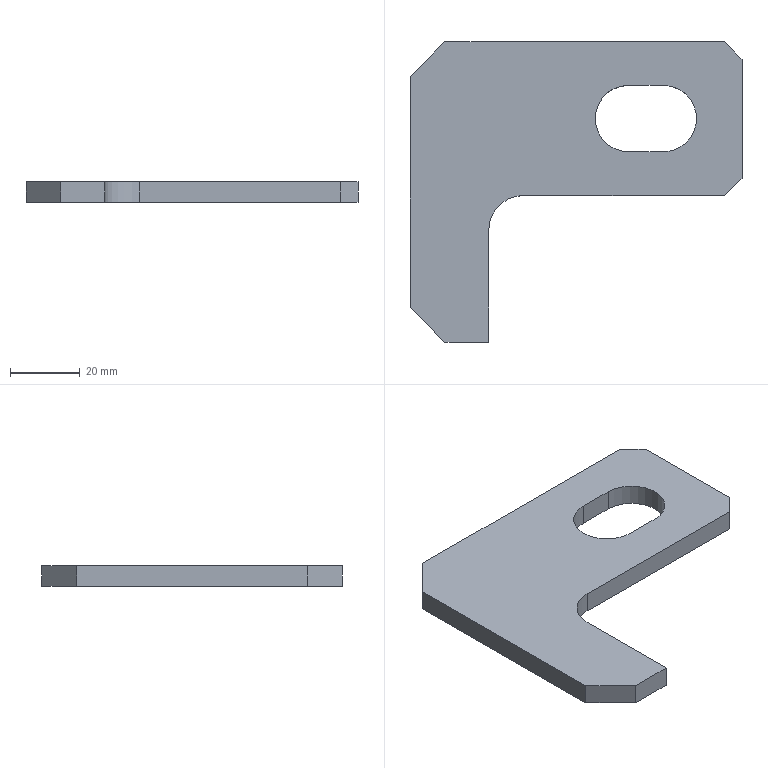Part | STEP file | 筋Plate-100×50-5 | 1 solid | 18 faces | box 95 x 86 x 6 mm | volume 27288 mm3 | plane 14 | cylinder 4 | commonest cylinder face diameters 19 x3 20 x1
STEP:
#1=CARTESIAN_POINT('',(0.,0.,0.));
#2=DIRECTION('',(0.,0.,1.));
#3=DIRECTION('',(1.,0.,0.));
#4=AXIS2_PLACEMENT_3D('',#1,#2,#3);
#5=CARTESIAN_POINT('',(15.,30.5,3.));
#6=VERTEX_POINT('',#5);
#7=CARTESIAN_POINT('',(15.,30.5,-3.));
#8=VERTEX_POINT('',#7);
#9=CARTESIAN_POINT('',(15.,30.5,-3.));
#10=DIRECTION('',(0.,0.,-1.));
#11=VECTOR('',#10,1.);
#12=LINE('',#9,#11);
#13=CARTESIAN_POINT('',(15.,21.,-3.));
#14=DIRECTION('',(0.,0.,-1.));
#15=DIRECTION('',(-1.,0.,0.));
#16=AXIS2_PLACEMENT_3D('',#13,#14,#15);
#17=CYLINDRICAL_SURFACE('',#16,9.5);
#18=CARTESIAN_POINT('',(1.571,0.));
#19=DIRECTION('',(0.,1.));
#20=VECTOR('',#19,1.);
#21=LINE('',#18,#20);
#22=(GEOMETRIC_REPRESENTATION_CONTEXT(2)PARAMETRIC_REPRESENTATION_CONTEXT()REPRESENTATION_CONTEXT('',''));
#23=DEFINITIONAL_REPRESENTATION('',(#21),#22);
#24=PCURVE('',#17,#23);
#25=CARTESIAN_POINT('',(15.,30.5,-3.));
#26=DIRECTION('',(0.,1.,0.));
#27=DIRECTION('',(-1.,0.,0.));
#28=AXIS2_PLACEMENT_3D('',#25,#26,#27);
#29=PLANE('',#28);
#30=CARTESIAN_POINT('',(0.,0.));
#31=DIRECTION('',(0.,-1.));
#32=VECTOR('',#31,1.);
#33=LINE('',#30,#32);
#34=(GEOMETRIC_REPRESENTATION_CONTEXT(2)PARAMETRIC_REPRESENTATION_CONTEXT()REPRESENTATION_CONTEXT('',''));
#35=DEFINITIONAL_REPRESENTATION('',(#33),#34);
#36=PCURVE('',#29,#35);
#37=SURFACE_CURVE('',#12,(#24,#36),.PCURVE_S1.);
#38=EDGE_CURVE('',#6,#8,#37,.T.);
#39=ORIENTED_EDGE('',*,*,#38,.T.);
#40=CARTESIAN_POINT('',(5.5,21.,-3.));
#41=VERTEX_POINT('',#40);
#42=CARTESIAN_POINT('',(15.,21.,-3.));
#43=DIRECTION('',(0.,0.,-1.));
#44=DIRECTION('',(-1.,0.,0.));
#45=AXIS2_PLACEMENT_3D('',#42,#43,#44);
#46=CIRCLE('',#45,9.5);
#47=CARTESIAN_POINT('',(0.,0.));
#48=DIRECTION('',(1.,0.));
#49=VECTOR('',#48,1.);
#50=LINE('',#47,#49);
#51=(GEOMETRIC_REPRESENTATION_CONTEXT(2)PARAMETRIC_REPRESENTATION_CONTEXT()REPRESENTATION_CONTEXT('',''));
#52=DEFINITIONAL_REPRESENTATION('',(#50),#51);
#53=PCURVE('',#17,#52);
#54=CARTESIAN_POINT('',(0.,0.,-3.));
#55=DIRECTION('',(0.,0.,1.));
#56=DIRECTION('',(1.,0.,0.));
#57=AXIS2_PLACEMENT_3D('',#54,#55,#56);
#58=PLANE('',#57);
#59=CARTESIAN_POINT('',(5.5,21.));
#60=CARTESIAN_POINT('',(5.5,37.454));
#61=CARTESIAN_POINT('',(19.75,29.227));
#62=CARTESIAN_POINT('',(34.,21.));
#63=CARTESIAN_POINT('',(19.75,12.773));
#64=CARTESIAN_POINT('',(5.5,4.546));
#65=CARTESIAN_POINT('',(5.5,21.));
#66=(BOUNDED_CURVE()B_SPLINE_CURVE(2,(#59,#60,#61,#62,#63,#64,#65),.UNSPECIFIED.,.T.,.F.)B_SPLINE_CURVE_WITH_KNOTS((1,2,2,2,2,1),(-2.094,0.,2.094,4.189,6.283,8.378),.UNSPECIFIED.)CURVE()GEOMETRIC_REPRESENTATION_ITEM()RATIONAL_B_SPLINE_CURVE((1.,0.5,1.,0.5,1.,0.5,1.))REPRESENTATION_ITEM(''));
#67=(GEOMETRIC_REPRESENTATION_CONTEXT(2)PARAMETRIC_REPRESENTATION_CONTEXT()REPRESENTATION_CONTEXT('',''));
#68=DEFINITIONAL_REPRESENTATION('',(#66),#67);
#69=PCURVE('',#58,#68);
#70=SURFACE_CURVE('',#46,(#53,#69),.PCURVE_S1.);
#71=EDGE_CURVE('',#41,#8,#70,.T.);
#72=ORIENTED_EDGE('',*,*,#71,.F.);
#73=CARTESIAN_POINT('',(5.5,21.,3.));
#74=VERTEX_POINT('',#73);
#75=CARTESIAN_POINT('',(5.5,21.,-3.));
#76=DIRECTION('',(0.,0.,-1.));
#77=VECTOR('',#76,1.);
#78=LINE('',#75,#77);
#79=CARTESIAN_POINT('',(0.,0.));
#80=DIRECTION('',(0.,1.));
#81=VECTOR('',#80,1.);
#82=LINE('',#79,#81);
#83=(GEOMETRIC_REPRESENTATION_CONTEXT(2)PARAMETRIC_REPRESENTATION_CONTEXT()REPRESENTATION_CONTEXT('',''));
#84=DEFINITIONAL_REPRESENTATION('',(#82),#83);
#85=PCURVE('',#17,#84);
#86=CARTESIAN_POINT('',(15.,21.,-3.));
#87=DIRECTION('',(0.,0.,-1.));
#88=DIRECTION('',(-1.,0.,0.));
#89=AXIS2_PLACEMENT_3D('',#86,#87,#88);
#90=CYLINDRICAL_SURFACE('',#89,9.5);
#91=CARTESIAN_POINT('',(6.283,0.));
#92=DIRECTION('',(0.,1.));
#93=VECTOR('',#92,1.);
#94=LINE('',#91,#93);
#95=(GEOMETRIC_REPRESENTATION_CONTEXT(2)PARAMETRIC_REPRESENTATION_CONTEXT()REPRESENTATION_CONTEXT('',''));
#96=DEFINITIONAL_REPRESENTATION('',(#94),#95);
#97=PCURVE('',#90,#96);
#98=SURFACE_CURVE('',#78,(#85,#97),.PCURVE_S1.);
#99=EDGE_CURVE('',#74,#41,#98,.T.);
#100=ORIENTED_EDGE('',*,*,#99,.F.);
#101=CARTESIAN_POINT('',(15.,21.,3.));
#102=DIRECTION('',(0.,0.,1.));
#103=DIRECTION('',(1.,0.,0.));
#104=AXIS2_PLACEMENT_3D('',#101,#102,#103);
#105=CIRCLE('',#104,9.5);
#106=CARTESIAN_POINT('',(3.142,-6.));
#107=DIRECTION('',(-1.,0.));
#108=VECTOR('',#107,1.);
#109=LINE('',#106,#108);
#110=(GEOMETRIC_REPRESENTATION_CONTEXT(2)PARAMETRIC_REPRESENTATION_CONTEXT()REPRESENTATION_CONTEXT('',''));
#111=DEFINITIONAL_REPRESENTATION('',(#109),#110);
#112=PCURVE('',#17,#111);
#113=CARTESIAN_POINT('',(0.,0.,3.));
#114=DIRECTION('',(0.,0.,1.));
#115=DIRECTION('',(1.,0.,0.));
#116=AXIS2_PLACEMENT_3D('',#113,#114,#115);
#117=PLANE('',#116);
#118=CARTESIAN_POINT('',(15.,21.));
#119=DIRECTION('',(1.,0.));
#120=AXIS2_PLACEMENT_2D('',#118,#119);
#121=CIRCLE('',#120,9.5);
#122=(GEOMETRIC_REPRESENTATION_CONTEXT(2)PARAMETRIC_REPRESENTATION_CONTEXT()REPRESENTATION_CONTEXT('',''));
#123=DEFINITIONAL_REPRESENTATION('',(#121),#122);
#124=PCURVE('',#117,#123);
#125=SURFACE_CURVE('',#105,(#112,#124),.PCURVE_S1.);
#126=EDGE_CURVE('',#6,#74,#125,.T.);
#127=ORIENTED_EDGE('',*,*,#126,.F.);
#128=EDGE_LOOP('',(#39,#72,#100,#127));
#129=FACE_BOUND('',#128,.F.);
#130=ADVANCED_FACE('',(#129),#17,.F.);
#131=CARTESIAN_POINT('',(47.5,38.,3.));
#132=VERTEX_POINT('',#131);
#133=CARTESIAN_POINT('',(47.5,4.,3.));
#134=VERTEX_POINT('',#133);
#135=CARTESIAN_POINT('',(47.5,0.,3.));
#136=DIRECTION('',(0.,-1.,0.));
#137=VECTOR('',#136,1.);
#138=LINE('',#135,#137);
#139=CARTESIAN_POINT('',(47.5,0.,3.));
#140=DIRECTION('',(1.,0.,0.));
#141=DIRECTION('',(0.,1.,0.));
#142=AXIS2_PLACEMENT_3D('',#139,#140,#141);
#143=PLANE('',#142);
#144=CARTESIAN_POINT('',(0.,0.));
#145=DIRECTION('',(-1.,0.));
#146=VECTOR('',#145,1.);
#147=LINE('',#144,#146);
#148=(GEOMETRIC_REPRESENTATION_CONTEXT(2)PARAMETRIC_REPRESENTATION_CONTEXT()REPRESENTATION_CONTEXT('',''));
#149=DEFINITIONAL_REPRESENTATION('',(#147),#148);
#150=PCURVE('',#143,#149);
#151=CARTESIAN_POINT('',(47.5,0.));
#152=DIRECTION('',(0.,-1.));
#153=VECTOR('',#152,1.);
#154=LINE('',#151,#153);
#155=(GEOMETRIC_REPRESENTATION_CONTEXT(2)PARAMETRIC_REPRESENTATION_CONTEXT()REPRESENTATION_CONTEXT('',''));
#156=DEFINITIONAL_REPRESENTATION('',(#154),#155);
#157=PCURVE('',#117,#156);
#158=SURFACE_CURVE('',#138,(#150,#157),.PCURVE_S1.);
#159=EDGE_CURVE('',#132,#134,#158,.T.);
#160=ORIENTED_EDGE('',*,*,#159,.T.);
#161=CARTESIAN_POINT('',(47.5,4.,-3.));
#162=VERTEX_POINT('',#161);
#163=CARTESIAN_POINT('',(47.5,4.,-3.));
#164=DIRECTION('',(0.,0.,-1.));
#165=VECTOR('',#164,1.);
#166=LINE('',#163,#165);
#167=CARTESIAN_POINT('',(4.,-6.));
#168=DIRECTION('',(0.,-1.));
#169=VECTOR('',#168,1.);
#170=LINE('',#167,#169);
#171=(GEOMETRIC_REPRESENTATION_CONTEXT(2)PARAMETRIC_REPRESENTATION_CONTEXT()REPRESENTATION_CONTEXT('',''));
#172=DEFINITIONAL_REPRESENTATION('',(#170),#171);
#173=PCURVE('',#143,#172);
#174=CARTESIAN_POINT('',(42.5,-1.,-3.));
#175=DIRECTION('',(0.7071,-0.7071,0.));
#176=DIRECTION('',(0.,0.,-1.));
#177=AXIS2_PLACEMENT_3D('',#174,#175,#176);
#178=PLANE('',#177);
#179=CARTESIAN_POINT('',(0.,7.071));
#180=DIRECTION('',(1.,0.));
#181=VECTOR('',#180,1.);
#182=LINE('',#179,#181);
#183=(GEOMETRIC_REPRESENTATION_CONTEXT(2)PARAMETRIC_REPRESENTATION_CONTEXT()REPRESENTATION_CONTEXT('',''));
#184=DEFINITIONAL_REPRESENTATION('',(#182),#183);
#185=PCURVE('',#178,#184);
#186=SURFACE_CURVE('',#166,(#173,#185),.PCURVE_S1.);
#187=EDGE_CURVE('',#134,#162,#186,.T.);
#188=ORIENTED_EDGE('',*,*,#187,.T.);
#189=CARTESIAN_POINT('',(47.5,38.,-3.));
#190=VERTEX_POINT('',#189);
#191=CARTESIAN_POINT('',(47.5,0.,-3.));
#192=DIRECTION('',(0.,-1.,0.));
#193=VECTOR('',#192,1.);
#194=LINE('',#191,#193);
#195=CARTESIAN_POINT('',(0.,-6.));
#196=DIRECTION('',(-1.,0.));
#197=VECTOR('',#196,1.);
#198=LINE('',#195,#197);
#199=(GEOMETRIC_REPRESENTATION_CONTEXT(2)PARAMETRIC_REPRESENTATION_CONTEXT()REPRESENTATION_CONTEXT('',''));
#200=DEFINITIONAL_REPRESENTATION('',(#198),#199);
#201=PCURVE('',#143,#200);
#202=CARTESIAN_POINT('',(47.5,0.));
#203=DIRECTION('',(0.,-1.));
#204=VECTOR('',#203,1.);
#205=LINE('',#202,#204);
#206=(GEOMETRIC_REPRESENTATION_CONTEXT(2)PARAMETRIC_REPRESENTATION_CONTEXT()REPRESENTATION_CONTEXT('',''));
#207=DEFINITIONAL_REPRESENTATION('',(#205),#206);
#208=PCURVE('',#58,#207);
#209=SURFACE_CURVE('',#194,(#201,#208),.PCURVE_S1.);
#210=EDGE_CURVE('',#190,#162,#209,.T.);
#211=ORIENTED_EDGE('',*,*,#210,.F.);
#212=CARTESIAN_POINT('',(47.5,38.,3.));
#213=DIRECTION('',(0.,0.,1.));
#214=VECTOR('',#213,1.);
#215=LINE('',#212,#214);
#216=CARTESIAN_POINT('',(38.,0.));
#217=DIRECTION('',(0.,1.));
#218=VECTOR('',#217,1.);
#219=LINE('',#216,#218);
#220=(GEOMETRIC_REPRESENTATION_CONTEXT(2)PARAMETRIC_REPRESENTATION_CONTEXT()REPRESENTATION_CONTEXT('',''));
#221=DEFINITIONAL_REPRESENTATION('',(#219),#220);
#222=PCURVE('',#143,#221);
#223=CARTESIAN_POINT('',(42.5,43.,3.));
#224=DIRECTION('',(-0.7071,-0.7071,0.));
#225=DIRECTION('',(0.,0.,-1.));
#226=AXIS2_PLACEMENT_3D('',#223,#224,#225);
#227=PLANE('',#226);
#228=CARTESIAN_POINT('',(0.,7.071));
#229=DIRECTION('',(-1.,0.));
#230=VECTOR('',#229,1.);
#231=LINE('',#228,#230);
#232=(GEOMETRIC_REPRESENTATION_CONTEXT(2)PARAMETRIC_REPRESENTATION_CONTEXT()REPRESENTATION_CONTEXT('',''));
#233=DEFINITIONAL_REPRESENTATION('',(#231),#232);
#234=PCURVE('',#227,#233);
#235=SURFACE_CURVE('',#215,(#222,#234),.PCURVE_S1.);
#236=EDGE_CURVE('',#190,#132,#235,.T.);
#237=ORIENTED_EDGE('',*,*,#236,.T.);
#238=EDGE_LOOP('',(#160,#188,#211,#237));
#239=FACE_BOUND('',#238,.T.);
#240=ADVANCED_FACE('',(#239),#143,.T.);
#241=CARTESIAN_POINT('',(-37.5,43.,3.));
#242=VERTEX_POINT('',#241);
#243=CARTESIAN_POINT('',(42.5,43.,3.));
#244=VERTEX_POINT('',#243);
#245=CARTESIAN_POINT('',(0.,43.,3.));
#246=DIRECTION('',(1.,0.,0.));
#247=VECTOR('',#246,1.);
#248=LINE('',#245,#247);
#249=CARTESIAN_POINT('',(0.,43.,3.));
#250=DIRECTION('',(0.,1.,0.));
#251=DIRECTION('',(0.,0.,1.));
#252=AXIS2_PLACEMENT_3D('',#249,#250,#251);
#253=PLANE('',#252);
#254=CARTESIAN_POINT('',(0.,0.));
#255=DIRECTION('',(0.,1.));
#256=VECTOR('',#255,1.);
#257=LINE('',#254,#256);
#258=(GEOMETRIC_REPRESENTATION_CONTEXT(2)PARAMETRIC_REPRESENTATION_CONTEXT()REPRESENTATION_CONTEXT('',''));
#259=DEFINITIONAL_REPRESENTATION('',(#257),#258);
#260=PCURVE('',#253,#259);
#261=CARTESIAN_POINT('',(0.,43.));
#262=DIRECTION('',(1.,0.));
#263=VECTOR('',#262,1.);
#264=LINE('',#261,#263);
#265=(GEOMETRIC_REPRESENTATION_CONTEXT(2)PARAMETRIC_REPRESENTATION_CONTEXT()REPRESENTATION_CONTEXT('',''));
#266=DEFINITIONAL_REPRESENTATION('',(#264),#265);
#267=PCURVE('',#117,#266);
#268=SURFACE_CURVE('',#248,(#260,#267),.PCURVE_S1.);
#269=EDGE_CURVE('',#242,#244,#268,.T.);
#270=ORIENTED_EDGE('',*,*,#269,.T.);
#271=CARTESIAN_POINT('',(42.5,43.,-3.));
#272=VERTEX_POINT('',#271);
#273=CARTESIAN_POINT('',(42.5,43.,3.));
#274=DIRECTION('',(0.,0.,-1.));
#275=VECTOR('',#274,1.);
#276=LINE('',#273,#275);
#277=CARTESIAN_POINT('',(0.,42.5));
#278=DIRECTION('',(-1.,0.));
#279=VECTOR('',#278,1.);
#280=LINE('',#277,#279);
#281=(GEOMETRIC_REPRESENTATION_CONTEXT(2)PARAMETRIC_REPRESENTATION_CONTEXT()REPRESENTATION_CONTEXT('',''));
#282=DEFINITIONAL_REPRESENTATION('',(#280),#281);
#283=PCURVE('',#253,#282);
#284=CARTESIAN_POINT('',(0.,0.));
#285=DIRECTION('',(1.,0.));
#286=VECTOR('',#285,1.);
#287=LINE('',#284,#286);
#288=(GEOMETRIC_REPRESENTATION_CONTEXT(2)PARAMETRIC_REPRESENTATION_CONTEXT()REPRESENTATION_CONTEXT('',''));
#289=DEFINITIONAL_REPRESENTATION('',(#287),#288);
#290=PCURVE('',#227,#289);
#291=SURFACE_CURVE('',#276,(#283,#290),.PCURVE_S1.);
#292=EDGE_CURVE('',#244,#272,#291,.T.);
#293=ORIENTED_EDGE('',*,*,#292,.T.);
#294=CARTESIAN_POINT('',(-37.5,43.,-3.));
#295=VERTEX_POINT('',#294);
#296=CARTESIAN_POINT('',(0.,43.,-3.));
#297=DIRECTION('',(1.,0.,0.));
#298=VECTOR('',#297,1.);
#299=LINE('',#296,#298);
#300=CARTESIAN_POINT('',(-6.,0.));
#301=DIRECTION('',(0.,1.));
#302=VECTOR('',#301,1.);
#303=LINE('',#300,#302);
#304=(GEOMETRIC_REPRESENTATION_CONTEXT(2)PARAMETRIC_REPRESENTATION_CONTEXT()REPRESENTATION_CONTEXT('',''));
#305=DEFINITIONAL_REPRESENTATION('',(#303),#304);
#306=PCURVE('',#253,#305);
#307=CARTESIAN_POINT('',(0.,43.));
#308=DIRECTION('',(1.,0.));
#309=VECTOR('',#308,1.);
#310=LINE('',#307,#309);
#311=(GEOMETRIC_REPRESENTATION_CONTEXT(2)PARAMETRIC_REPRESENTATION_CONTEXT()REPRESENTATION_CONTEXT('',''));
#312=DEFINITIONAL_REPRESENTATION('',(#310),#311);
#313=PCURVE('',#58,#312);
#314=SURFACE_CURVE('',#299,(#306,#313),.PCURVE_S1.);
#315=EDGE_CURVE('',#295,#272,#314,.T.);
#316=ORIENTED_EDGE('',*,*,#315,.F.);
#317=CARTESIAN_POINT('',(-37.5,43.,3.));
#318=DIRECTION('',(0.,0.,1.));
#319=VECTOR('',#318,1.);
#320=LINE('',#317,#319);
#321=CARTESIAN_POINT('',(0.,-37.5));
#322=DIRECTION('',(1.,0.));
#323=VECTOR('',#322,1.);
#324=LINE('',#321,#323);
#325=(GEOMETRIC_REPRESENTATION_CONTEXT(2)PARAMETRIC_REPRESENTATION_CONTEXT()REPRESENTATION_CONTEXT('',''));
#326=DEFINITIONAL_REPRESENTATION('',(#324),#325);
#327=PCURVE('',#253,#326);
#328=CARTESIAN_POINT('',(-47.5,33.,3.));
#329=DIRECTION('',(-0.7071,0.7071,0.));
#330=DIRECTION('',(0.,0.,1.));
#331=AXIS2_PLACEMENT_3D('',#328,#329,#330);
#332=PLANE('',#331);
#333=CARTESIAN_POINT('',(0.,14.142));
#334=DIRECTION('',(1.,0.));
#335=VECTOR('',#334,1.);
#336=LINE('',#333,#335);
#337=(GEOMETRIC_REPRESENTATION_CONTEXT(2)PARAMETRIC_REPRESENTATION_CONTEXT()REPRESENTATION_CONTEXT('',''));
#338=DEFINITIONAL_REPRESENTATION('',(#336),#337);
#339=PCURVE('',#332,#338);
#340=SURFACE_CURVE('',#320,(#327,#339),.PCURVE_S1.);
#341=EDGE_CURVE('',#295,#242,#340,.T.);
#342=ORIENTED_EDGE('',*,*,#341,.T.);
#343=EDGE_LOOP('',(#270,#293,#316,#342));
#344=FACE_BOUND('',#343,.T.);
#345=ADVANCED_FACE('',(#344),#253,.T.);
#346=CARTESIAN_POINT('',(-47.5,33.,-3.));
#347=VERTEX_POINT('',#346);
#348=CARTESIAN_POINT('',(-47.5,-33.,-3.));
#349=VERTEX_POINT('',#348);
#350=CARTESIAN_POINT('',(-47.5,0.,-3.));
#351=DIRECTION('',(0.,-1.,0.));
#352=VECTOR('',#351,1.);
#353=LINE('',#350,#352);
#354=CARTESIAN_POINT('',(-47.5,0.,3.));
#355=DIRECTION('',(1.,0.,0.));
#356=DIRECTION('',(0.,1.,0.));
#357=AXIS2_PLACEMENT_3D('',#354,#355,#356);
#358=PLANE('',#357);
#359=CARTESIAN_POINT('',(0.,-6.));
#360=DIRECTION('',(-1.,0.));
#361=VECTOR('',#360,1.);
#362=LINE('',#359,#361);
#363=(GEOMETRIC_REPRESENTATION_CONTEXT(2)PARAMETRIC_REPRESENTATION_CONTEXT()REPRESENTATION_CONTEXT('',''));
#364=DEFINITIONAL_REPRESENTATION('',(#362),#363);
#365=PCURVE('',#358,#364);
#366=CARTESIAN_POINT('',(-47.5,0.));
#367=DIRECTION('',(0.,-1.));
#368=VECTOR('',#367,1.);
#369=LINE('',#366,#368);
#370=(GEOMETRIC_REPRESENTATION_CONTEXT(2)PARAMETRIC_REPRESENTATION_CONTEXT()REPRESENTATION_CONTEXT('',''));
#371=DEFINITIONAL_REPRESENTATION('',(#369),#370);
#372=PCURVE('',#58,#371);
#373=SURFACE_CURVE('',#353,(#365,#372),.PCURVE_S1.);
#374=EDGE_CURVE('',#347,#349,#373,.T.);
#375=ORIENTED_EDGE('',*,*,#374,.T.);
#376=CARTESIAN_POINT('',(-47.5,-33.,3.));
#377=VERTEX_POINT('',#376);
#378=CARTESIAN_POINT('',(-47.5,-33.,3.));
#379=DIRECTION('',(0.,0.,1.));
#380=VECTOR('',#379,1.);
#381=LINE('',#378,#380);
#382=CARTESIAN_POINT('',(-33.,0.));
#383=DIRECTION('',(0.,1.));
#384=VECTOR('',#383,1.);
#385=LINE('',#382,#384);
#386=(GEOMETRIC_REPRESENTATION_CONTEXT(2)PARAMETRIC_REPRESENTATION_CONTEXT()REPRESENTATION_CONTEXT('',''));
#387=DEFINITIONAL_REPRESENTATION('',(#385),#386);
#388=PCURVE('',#358,#387);
#389=CARTESIAN_POINT('',(-37.5,-43.,3.));
#390=DIRECTION('',(0.7071,0.7071,0.));
#391=DIRECTION('',(0.,0.,-1.));
#392=AXIS2_PLACEMENT_3D('',#389,#390,#391);
#393=PLANE('',#392);
#394=CARTESIAN_POINT('',(0.,14.142));
#395=DIRECTION('',(-1.,0.));
#396=VECTOR('',#395,1.);
#397=LINE('',#394,#396);
#398=(GEOMETRIC_REPRESENTATION_CONTEXT(2)PARAMETRIC_REPRESENTATION_CONTEXT()REPRESENTATION_CONTEXT('',''));
#399=DEFINITIONAL_REPRESENTATION('',(#397),#398);
#400=PCURVE('',#393,#399);
#401=SURFACE_CURVE('',#381,(#388,#400),.PCURVE_S1.);
#402=EDGE_CURVE('',#349,#377,#401,.T.);
#403=ORIENTED_EDGE('',*,*,#402,.T.);
#404=CARTESIAN_POINT('',(-47.5,33.,3.));
#405=VERTEX_POINT('',#404);
#406=CARTESIAN_POINT('',(-47.5,0.,3.));
#407=DIRECTION('',(0.,-1.,0.));
#408=VECTOR('',#407,1.);
#409=LINE('',#406,#408);
#410=CARTESIAN_POINT('',(0.,0.));
#411=DIRECTION('',(-1.,0.));
#412=VECTOR('',#411,1.);
#413=LINE('',#410,#412);
#414=(GEOMETRIC_REPRESENTATION_CONTEXT(2)PARAMETRIC_REPRESENTATION_CONTEXT()REPRESENTATION_CONTEXT('',''));
#415=DEFINITIONAL_REPRESENTATION('',(#413),#414);
#416=PCURVE('',#358,#415);
#417=CARTESIAN_POINT('',(-47.5,0.));
#418=DIRECTION('',(0.,-1.));
#419=VECTOR('',#418,1.);
#420=LINE('',#417,#419);
#421=(GEOMETRIC_REPRESENTATION_CONTEXT(2)PARAMETRIC_REPRESENTATION_CONTEXT()REPRESENTATION_CONTEXT('',''));
#422=DEFINITIONAL_REPRESENTATION('',(#420),#421);
#423=PCURVE('',#117,#422);
#424=SURFACE_CURVE('',#409,(#416,#423),.PCURVE_S1.);
#425=EDGE_CURVE('',#405,#377,#424,.T.);
#426=ORIENTED_EDGE('',*,*,#425,.F.);
#427=CARTESIAN_POINT('',(-47.5,33.,-3.));
#428=DIRECTION('',(0.,0.,-1.));
#429=VECTOR('',#428,1.);
#430=LINE('',#427,#429);
#431=CARTESIAN_POINT('',(33.,-6.));
#432=DIRECTION('',(0.,-1.));
#433=VECTOR('',#432,1.);
#434=LINE('',#431,#433);
#435=(GEOMETRIC_REPRESENTATION_CONTEXT(2)PARAMETRIC_REPRESENTATION_CONTEXT()REPRESENTATION_CONTEXT('',''));
#436=DEFINITIONAL_REPRESENTATION('',(#434),#435);
#437=PCURVE('',#358,#436);
#438=CARTESIAN_POINT('',(-6.,0.));
#439=DIRECTION('',(-1.,0.));
#440=VECTOR('',#439,1.);
#441=LINE('',#438,#440);
#442=(GEOMETRIC_REPRESENTATION_CONTEXT(2)PARAMETRIC_REPRESENTATION_CONTEXT()REPRESENTATION_CONTEXT('',''));
#443=DEFINITIONAL_REPRESENTATION('',(#441),#442);
#444=PCURVE('',#332,#443);
#445=SURFACE_CURVE('',#430,(#437,#444),.PCURVE_S1.);
#446=EDGE_CURVE('',#405,#347,#445,.T.);
#447=ORIENTED_EDGE('',*,*,#446,.T.);
#448=EDGE_LOOP('',(#375,#403,#426,#447));
#449=FACE_BOUND('',#448,.T.);
#450=ADVANCED_FACE('',(#449),#358,.F.);
#451=CARTESIAN_POINT('',(-37.5,-43.,3.));
#452=VERTEX_POINT('',#451);
#453=CARTESIAN_POINT('',(-25.,-43.,3.));
#454=VERTEX_POINT('',#453);
#455=CARTESIAN_POINT('',(0.,-43.,3.));
#456=DIRECTION('',(1.,0.,0.));
#457=VECTOR('',#456,1.);
#458=LINE('',#455,#457);
#459=CARTESIAN_POINT('',(0.,-43.,3.));
#460=DIRECTION('',(0.,1.,0.));
#461=DIRECTION('',(0.,0.,1.));
#462=AXIS2_PLACEMENT_3D('',#459,#460,#461);
#463=PLANE('',#462);
#464=CARTESIAN_POINT('',(0.,0.));
#465=DIRECTION('',(0.,1.));
#466=VECTOR('',#465,1.);
#467=LINE('',#464,#466);
#468=(GEOMETRIC_REPRESENTATION_CONTEXT(2)PARAMETRIC_REPRESENTATION_CONTEXT()REPRESENTATION_CONTEXT('',''));
#469=DEFINITIONAL_REPRESENTATION('',(#467),#468);
#470=PCURVE('',#463,#469);
#471=CARTESIAN_POINT('',(0.,-43.));
#472=DIRECTION('',(1.,0.));
#473=VECTOR('',#472,1.);
#474=LINE('',#471,#473);
#475=(GEOMETRIC_REPRESENTATION_CONTEXT(2)PARAMETRIC_REPRESENTATION_CONTEXT()REPRESENTATION_CONTEXT('',''));
#476=DEFINITIONAL_REPRESENTATION('',(#474),#475);
#477=PCURVE('',#117,#476);
#478=SURFACE_CURVE('',#458,(#470,#477),.PCURVE_S1.);
#479=EDGE_CURVE('',#452,#454,#478,.T.);
#480=ORIENTED_EDGE('',*,*,#479,.F.);
#481=CARTESIAN_POINT('',(-37.5,-43.,-3.));
#482=VERTEX_POINT('',#481);
#483=CARTESIAN_POINT('',(-37.5,-43.,3.));
#484=DIRECTION('',(0.,0.,-1.));
#485=VECTOR('',#484,1.);
#486=LINE('',#483,#485);
#487=CARTESIAN_POINT('',(0.,-37.5));
#488=DIRECTION('',(-1.,0.));
#489=VECTOR('',#488,1.);
#490=LINE('',#487,#489);
#491=(GEOMETRIC_REPRESENTATION_CONTEXT(2)PARAMETRIC_REPRESENTATION_CONTEXT()REPRESENTATION_CONTEXT('',''));
#492=DEFINITIONAL_REPRESENTATION('',(#490),#491);
#493=PCURVE('',#463,#492);
#494=CARTESIAN_POINT('',(0.,0.));
#495=DIRECTION('',(1.,0.));
#496=VECTOR('',#495,1.);
#497=LINE('',#494,#496);
#498=(GEOMETRIC_REPRESENTATION_CONTEXT(2)PARAMETRIC_REPRESENTATION_CONTEXT()REPRESENTATION_CONTEXT('',''));
#499=DEFINITIONAL_REPRESENTATION('',(#497),#498);
#500=PCURVE('',#393,#499);
#501=SURFACE_CURVE('',#486,(#493,#500),.PCURVE_S1.);
#502=EDGE_CURVE('',#452,#482,#501,.T.);
#503=ORIENTED_EDGE('',*,*,#502,.T.);
#504=CARTESIAN_POINT('',(-25.,-43.,-3.));
#505=VERTEX_POINT('',#504);
#506=CARTESIAN_POINT('',(0.,-43.,-3.));
#507=DIRECTION('',(1.,0.,0.));
#508=VECTOR('',#507,1.);
#509=LINE('',#506,#508);
#510=CARTESIAN_POINT('',(-6.,0.));
#511=DIRECTION('',(0.,1.));
#512=VECTOR('',#511,1.);
#513=LINE('',#510,#512);
#514=(GEOMETRIC_REPRESENTATION_CONTEXT(2)PARAMETRIC_REPRESENTATION_CONTEXT()REPRESENTATION_CONTEXT('',''));
#515=DEFINITIONAL_REPRESENTATION('',(#513),#514);
#516=PCURVE('',#463,#515);
#517=CARTESIAN_POINT('',(0.,-43.));
#518=DIRECTION('',(1.,0.));
#519=VECTOR('',#518,1.);
#520=LINE('',#517,#519);
#521=(GEOMETRIC_REPRESENTATION_CONTEXT(2)PARAMETRIC_REPRESENTATION_CONTEXT()REPRESENTATION_CONTEXT('',''));
#522=DEFINITIONAL_REPRESENTATION('',(#520),#521);
#523=PCURVE('',#58,#522);
#524=SURFACE_CURVE('',#509,(#516,#523),.PCURVE_S1.);
#525=EDGE_CURVE('',#482,#505,#524,.T.);
#526=ORIENTED_EDGE('',*,*,#525,.T.);
#527=CARTESIAN_POINT('',(-25.,-43.,-3.));
#528=DIRECTION('',(0.,0.,1.));
#529=VECTOR('',#528,1.);
#530=LINE('',#527,#529);
#531=CARTESIAN_POINT('',(-6.,-25.));
#532=DIRECTION('',(1.,0.));
#533=VECTOR('',#532,1.);
#534=LINE('',#531,#533);
#535=(GEOMETRIC_REPRESENTATION_CONTEXT(2)PARAMETRIC_REPRESENTATION_CONTEXT()REPRESENTATION_CONTEXT('',''));
#536=DEFINITIONAL_REPRESENTATION('',(#534),#535);
#537=PCURVE('',#463,#536);
#538=CARTESIAN_POINT('',(-25.,-43.,-3.));
#539=DIRECTION('',(-1.,0.,0.));
#540=DIRECTION('',(0.,0.,1.));
#541=AXIS2_PLACEMENT_3D('',#538,#539,#540);
#542=PLANE('',#541);
#543=CARTESIAN_POINT('',(0.,0.));
#544=DIRECTION('',(1.,0.));
#545=VECTOR('',#544,1.);
#546=LINE('',#543,#545);
#547=(GEOMETRIC_REPRESENTATION_CONTEXT(2)PARAMETRIC_REPRESENTATION_CONTEXT()REPRESENTATION_CONTEXT('',''));
#548=DEFINITIONAL_REPRESENTATION('',(#546),#547);
#549=PCURVE('',#542,#548);
#550=SURFACE_CURVE('',#530,(#537,#549),.PCURVE_S1.);
#551=EDGE_CURVE('',#505,#454,#550,.T.);
#552=ORIENTED_EDGE('',*,*,#551,.T.);
#553=EDGE_LOOP('',(#480,#503,#526,#552));
#554=FACE_BOUND('',#553,.T.);
#555=ADVANCED_FACE('',(#554),#463,.F.);
#556=ORIENTED_EDGE('',*,*,#126,.F.);
#557=CARTESIAN_POINT('',(25.,30.5,3.));
#558=VERTEX_POINT('',#557);
#559=CARTESIAN_POINT('',(0.,30.5,3.));
#560=DIRECTION('',(-1.,0.,0.));
#561=VECTOR('',#560,1.);
#562=LINE('',#559,#561);
#563=CARTESIAN_POINT('',(0.,30.5));
#564=DIRECTION('',(-1.,0.));
#565=VECTOR('',#564,1.);
#566=LINE('',#563,#565);
#567=(GEOMETRIC_REPRESENTATION_CONTEXT(2)PARAMETRIC_REPRESENTATION_CONTEXT()REPRESENTATION_CONTEXT('',''));
#568=DEFINITIONAL_REPRESENTATION('',(#566),#567);
#569=PCURVE('',#117,#568);
#570=CARTESIAN_POINT('',(15.,6.));
#571=DIRECTION('',(1.,0.));
#572=VECTOR('',#571,1.);
#573=LINE('',#570,#572);
#574=(GEOMETRIC_REPRESENTATION_CONTEXT(2)PARAMETRIC_REPRESENTATION_CONTEXT()REPRESENTATION_CONTEXT('',''));
#575=DEFINITIONAL_REPRESENTATION('',(#573),#574);
#576=PCURVE('',#29,#575);
#577=SURFACE_CURVE('',#562,(#569,#576),.PCURVE_S1.);
#578=EDGE_CURVE('',#558,#6,#577,.T.);
#579=ORIENTED_EDGE('',*,*,#578,.F.);
#580=CARTESIAN_POINT('',(25.,11.5,3.));
#581=VERTEX_POINT('',#580);
#582=CARTESIAN_POINT('',(25.,21.,3.));
#583=DIRECTION('',(0.,0.,1.));
#584=DIRECTION('',(1.,0.,0.));
#585=AXIS2_PLACEMENT_3D('',#582,#583,#584);
#586=CIRCLE('',#585,9.5);
#587=CARTESIAN_POINT('',(25.,21.));
#588=DIRECTION('',(1.,0.));
#589=AXIS2_PLACEMENT_2D('',#587,#588);
#590=CIRCLE('',#589,9.5);
#591=(GEOMETRIC_REPRESENTATION_CONTEXT(2)PARAMETRIC_REPRESENTATION_CONTEXT()REPRESENTATION_CONTEXT('',''));
#592=DEFINITIONAL_REPRESENTATION('',(#590),#591);
#593=PCURVE('',#117,#592);
#594=CARTESIAN_POINT('',(25.,21.,-3.));
#595=DIRECTION('',(0.,0.,-1.));
#596=DIRECTION('',(-1.,0.,0.));
#597=AXIS2_PLACEMENT_3D('',#594,#595,#596);
#598=CYLINDRICAL_SURFACE('',#597,9.5);
#599=CARTESIAN_POINT('',(9.425,-6.));
#600=DIRECTION('',(-1.,0.));
#601=VECTOR('',#600,1.);
#602=LINE('',#599,#601);
#603=(GEOMETRIC_REPRESENTATION_CONTEXT(2)PARAMETRIC_REPRESENTATION_CONTEXT()REPRESENTATION_CONTEXT('',''));
#604=DEFINITIONAL_REPRESENTATION('',(#602),#603);
#605=PCURVE('',#598,#604);
#606=SURFACE_CURVE('',#586,(#593,#605),.PCURVE_S1.);
#607=EDGE_CURVE('',#581,#558,#606,.T.);
#608=ORIENTED_EDGE('',*,*,#607,.F.);
#609=CARTESIAN_POINT('',(15.,11.5,3.));
#610=VERTEX_POINT('',#609);
#611=CARTESIAN_POINT('',(0.,11.5,3.));
#612=DIRECTION('',(1.,0.,0.));
#613=VECTOR('',#612,1.);
#614=LINE('',#611,#613);
#615=CARTESIAN_POINT('',(0.,11.5));
#616=DIRECTION('',(1.,0.));
#617=VECTOR('',#616,1.);
#618=LINE('',#615,#617);
#619=(GEOMETRIC_REPRESENTATION_CONTEXT(2)PARAMETRIC_REPRESENTATION_CONTEXT()REPRESENTATION_CONTEXT('',''));
#620=DEFINITIONAL_REPRESENTATION('',(#618),#619);
#621=PCURVE('',#117,#620);
#622=CARTESIAN_POINT('',(15.,11.5,-3.));
#623=DIRECTION('',(0.,-1.,0.));
#624=DIRECTION('',(1.,0.,0.));
#625=AXIS2_PLACEMENT_3D('',#622,#623,#624);
#626=PLANE('',#625);
#627=CARTESIAN_POINT('',(-15.,6.));
#628=DIRECTION('',(1.,0.));
#629=VECTOR('',#628,1.);
#630=LINE('',#627,#629);
#631=(GEOMETRIC_REPRESENTATION_CONTEXT(2)PARAMETRIC_REPRESENTATION_CONTEXT()REPRESENTATION_CONTEXT('',''));
#632=DEFINITIONAL_REPRESENTATION('',(#630),#631);
#633=PCURVE('',#626,#632);
#634=SURFACE_CURVE('',#614,(#621,#633),.PCURVE_S1.);
#635=EDGE_CURVE('',#610,#581,#634,.T.);
#636=ORIENTED_EDGE('',*,*,#635,.F.);
#637=CARTESIAN_POINT('',(15.,21.,3.));
#638=DIRECTION('',(0.,0.,1.));
#639=DIRECTION('',(1.,0.,0.));
#640=AXIS2_PLACEMENT_3D('',#637,#638,#639);
#641=CIRCLE('',#640,9.5);
#642=CARTESIAN_POINT('',(15.,21.));
#643=DIRECTION('',(1.,0.));
#644=AXIS2_PLACEMENT_2D('',#642,#643);
#645=CIRCLE('',#644,9.5);
#646=(GEOMETRIC_REPRESENTATION_CONTEXT(2)PARAMETRIC_REPRESENTATION_CONTEXT()REPRESENTATION_CONTEXT('',''));
#647=DEFINITIONAL_REPRESENTATION('',(#645),#646);
#648=PCURVE('',#117,#647);
#649=CARTESIAN_POINT('',(9.425,-6.));
#650=DIRECTION('',(-1.,0.));
#651=VECTOR('',#650,1.);
#652=LINE('',#649,#651);
#653=(GEOMETRIC_REPRESENTATION_CONTEXT(2)PARAMETRIC_REPRESENTATION_CONTEXT()REPRESENTATION_CONTEXT('',''));
#654=DEFINITIONAL_REPRESENTATION('',(#652),#653);
#655=PCURVE('',#90,#654);
#656=SURFACE_CURVE('',#641,(#648,#655),.PCURVE_S1.);
#657=EDGE_CURVE('',#74,#610,#656,.T.);
#658=ORIENTED_EDGE('',*,*,#657,.F.);
#659=EDGE_LOOP('',(#556,#579,#608,#636,#658));
#660=FACE_BOUND('',#659,.T.);
#661=CARTESIAN_POINT('',(42.5,-1.,3.));
#662=VERTEX_POINT('',#661);
#663=CARTESIAN_POINT('',(-15.,-1.,3.));
#664=VERTEX_POINT('',#663);
#665=CARTESIAN_POINT('',(47.5,-1.,3.));
#666=DIRECTION('',(-1.,0.,0.));
#667=VECTOR('',#666,1.);
#668=LINE('',#665,#667);
#669=CARTESIAN_POINT('',(47.5,-1.));
#670=DIRECTION('',(-1.,0.));
#671=VECTOR('',#670,1.);
#672=LINE('',#669,#671);
#673=(GEOMETRIC_REPRESENTATION_CONTEXT(2)PARAMETRIC_REPRESENTATION_CONTEXT()REPRESENTATION_CONTEXT('',''));
#674=DEFINITIONAL_REPRESENTATION('',(#672),#673);
#675=PCURVE('',#117,#674);
#676=CARTESIAN_POINT('',(47.5,-1.,-3.));
#677=DIRECTION('',(0.,1.,0.));
#678=DIRECTION('',(-1.,0.,0.));
#679=AXIS2_PLACEMENT_3D('',#676,#677,#678);
#680=PLANE('',#679);
#681=CARTESIAN_POINT('',(0.,6.));
#682=DIRECTION('',(1.,0.));
#683=VECTOR('',#682,1.);
#684=LINE('',#681,#683);
#685=(GEOMETRIC_REPRESENTATION_CONTEXT(2)PARAMETRIC_REPRESENTATION_CONTEXT()REPRESENTATION_CONTEXT('',''));
#686=DEFINITIONAL_REPRESENTATION('',(#684),#685);
#687=PCURVE('',#680,#686);
#688=SURFACE_CURVE('',#668,(#675,#687),.PCURVE_S1.);
#689=EDGE_CURVE('',#662,#664,#688,.T.);
#690=ORIENTED_EDGE('',*,*,#689,.F.);
#691=CARTESIAN_POINT('',(21.75,-21.75,3.));
#692=DIRECTION('',(0.7071,0.7071,0.));
#693=VECTOR('',#692,1.);
#694=LINE('',#691,#693);
#695=CARTESIAN_POINT('',(21.75,-21.75));
#696=DIRECTION('',(0.7071,0.7071));
#697=VECTOR('',#696,1.);
#698=LINE('',#695,#697);
#699=(GEOMETRIC_REPRESENTATION_CONTEXT(2)PARAMETRIC_REPRESENTATION_CONTEXT()REPRESENTATION_CONTEXT('',''));
#700=DEFINITIONAL_REPRESENTATION('',(#698),#699);
#701=PCURVE('',#117,#700);
#702=CARTESIAN_POINT('',(-6.,-29.345));
#703=DIRECTION('',(0.,1.));
#704=VECTOR('',#703,1.);
#705=LINE('',#702,#704);
#706=(GEOMETRIC_REPRESENTATION_CONTEXT(2)PARAMETRIC_REPRESENTATION_CONTEXT()REPRESENTATION_CONTEXT('',''));
#707=DEFINITIONAL_REPRESENTATION('',(#705),#706);
#708=PCURVE('',#178,#707);
#709=SURFACE_CURVE('',#694,(#701,#708),.PCURVE_S1.);
#710=EDGE_CURVE('',#662,#134,#709,.T.);
#711=ORIENTED_EDGE('',*,*,#710,.T.);
#712=ORIENTED_EDGE('',*,*,#159,.F.);
#713=CARTESIAN_POINT('',(42.75,42.75,3.));
#714=DIRECTION('',(-0.7071,0.7071,0.));
#715=VECTOR('',#714,1.);
#716=LINE('',#713,#715);
#717=CARTESIAN_POINT('',(42.75,42.75));
#718=DIRECTION('',(-0.7071,0.7071));
#719=VECTOR('',#718,1.);
#720=LINE('',#717,#719);
#721=(GEOMETRIC_REPRESENTATION_CONTEXT(2)PARAMETRIC_REPRESENTATION_CONTEXT()REPRESENTATION_CONTEXT('',''));
#722=DEFINITIONAL_REPRESENTATION('',(#720),#721);
#723=PCURVE('',#117,#722);
#724=CARTESIAN_POINT('',(0.,0.3536));
#725=DIRECTION('',(0.,-1.));
#726=VECTOR('',#725,1.);
#727=LINE('',#724,#726);
#728=(GEOMETRIC_REPRESENTATION_CONTEXT(2)PARAMETRIC_REPRESENTATION_CONTEXT()REPRESENTATION_CONTEXT('',''));
#729=DEFINITIONAL_REPRESENTATION('',(#727),#728);
#730=PCURVE('',#227,#729);
#731=SURFACE_CURVE('',#716,(#723,#730),.PCURVE_S1.);
#732=EDGE_CURVE('',#132,#244,#731,.T.);
#733=ORIENTED_EDGE('',*,*,#732,.T.);
#734=ORIENTED_EDGE('',*,*,#269,.F.);
#735=CARTESIAN_POINT('',(-40.25,40.25,3.));
#736=DIRECTION('',(-0.7071,-0.7071,0.));
#737=VECTOR('',#736,1.);
#738=LINE('',#735,#737);
#739=CARTESIAN_POINT('',(-40.25,40.25));
#740=DIRECTION('',(-0.7071,-0.7071));
#741=VECTOR('',#740,1.);
#742=LINE('',#739,#741);
#743=(GEOMETRIC_REPRESENTATION_CONTEXT(2)PARAMETRIC_REPRESENTATION_CONTEXT()REPRESENTATION_CONTEXT('',''));
#744=DEFINITIONAL_REPRESENTATION('',(#742),#743);
#745=PCURVE('',#117,#744);
#746=CARTESIAN_POINT('',(0.,10.253));
#747=DIRECTION('',(0.,-1.));
#748=VECTOR('',#747,1.);
#749=LINE('',#746,#748);
#750=(GEOMETRIC_REPRESENTATION_CONTEXT(2)PARAMETRIC_REPRESENTATION_CONTEXT()REPRESENTATION_CONTEXT('',''));
#751=DEFINITIONAL_REPRESENTATION('',(#749),#750);
#752=PCURVE('',#332,#751);
#753=SURFACE_CURVE('',#738,(#745,#752),.PCURVE_S1.);
#754=EDGE_CURVE('',#242,#405,#753,.T.);
#755=ORIENTED_EDGE('',*,*,#754,.T.);
#756=ORIENTED_EDGE('',*,*,#425,.T.);
#757=CARTESIAN_POINT('',(-40.25,-40.25,3.));
#758=DIRECTION('',(0.7071,-0.7071,0.));
#759=VECTOR('',#758,1.);
#760=LINE('',#757,#759);
#761=CARTESIAN_POINT('',(-40.25,-40.25));
#762=DIRECTION('',(0.7071,-0.7071));
#763=VECTOR('',#762,1.);
#764=LINE('',#761,#763);
#765=(GEOMETRIC_REPRESENTATION_CONTEXT(2)PARAMETRIC_REPRESENTATION_CONTEXT()REPRESENTATION_CONTEXT('',''));
#766=DEFINITIONAL_REPRESENTATION('',(#764),#765);
#767=PCURVE('',#117,#766);
#768=CARTESIAN_POINT('',(0.,3.889));
#769=DIRECTION('',(0.,-1.));
#770=VECTOR('',#769,1.);
#771=LINE('',#768,#770);
#772=(GEOMETRIC_REPRESENTATION_CONTEXT(2)PARAMETRIC_REPRESENTATION_CONTEXT()REPRESENTATION_CONTEXT('',''));
#773=DEFINITIONAL_REPRESENTATION('',(#771),#772);
#774=PCURVE('',#393,#773);
#775=SURFACE_CURVE('',#760,(#767,#774),.PCURVE_S1.);
#776=EDGE_CURVE('',#377,#452,#775,.T.);
#777=ORIENTED_EDGE('',*,*,#776,.T.);
#778=ORIENTED_EDGE('',*,*,#479,.T.);
#779=CARTESIAN_POINT('',(-25.,-11.,3.));
#780=VERTEX_POINT('',#779);
#781=CARTESIAN_POINT('',(-25.,-43.,3.));
#782=DIRECTION('',(0.,-1.,0.));
#783=VECTOR('',#782,1.);
#784=LINE('',#781,#783);
#785=CARTESIAN_POINT('',(-25.,-43.));
#786=DIRECTION('',(0.,-1.));
#787=VECTOR('',#786,1.);
#788=LINE('',#785,#787);
#789=(GEOMETRIC_REPRESENTATION_CONTEXT(2)PARAMETRIC_REPRESENTATION_CONTEXT()REPRESENTATION_CONTEXT('',''));
#790=DEFINITIONAL_REPRESENTATION('',(#788),#789);
#791=PCURVE('',#117,#790);
#792=CARTESIAN_POINT('',(6.,0.));
#793=DIRECTION('',(0.,-1.));
#794=VECTOR('',#793,1.);
#795=LINE('',#792,#794);
#796=(GEOMETRIC_REPRESENTATION_CONTEXT(2)PARAMETRIC_REPRESENTATION_CONTEXT()REPRESENTATION_CONTEXT('',''));
#797=DEFINITIONAL_REPRESENTATION('',(#795),#796);
#798=PCURVE('',#542,#797);
#799=SURFACE_CURVE('',#784,(#791,#798),.PCURVE_S1.);
#800=EDGE_CURVE('',#780,#454,#799,.T.);
#801=ORIENTED_EDGE('',*,*,#800,.F.);
#802=CARTESIAN_POINT('',(-15.,-11.,3.));
#803=DIRECTION('',(0.,0.,-1.));
#804=DIRECTION('',(1.,0.,0.));
#805=AXIS2_PLACEMENT_3D('',#802,#803,#804);
#806=CIRCLE('',#805,10.);
#807=CARTESIAN_POINT('',(-5.,-11.));
#808=CARTESIAN_POINT('',(-5.,-28.321));
#809=CARTESIAN_POINT('',(-20.,-19.66));
#810=CARTESIAN_POINT('',(-35.,-11.));
#811=CARTESIAN_POINT('',(-20.,-2.34));
#812=CARTESIAN_POINT('',(-5.,6.321));
#813=CARTESIAN_POINT('',(-5.,-11.));
#814=(BOUNDED_CURVE()B_SPLINE_CURVE(2,(#807,#808,#809,#810,#811,#812,#813),.UNSPECIFIED.,.T.,.F.)B_SPLINE_CURVE_WITH_KNOTS((1,2,2,2,2,1),(-2.094,0.,2.094,4.189,6.283,8.378),.UNSPECIFIED.)CURVE()GEOMETRIC_REPRESENTATION_ITEM()RATIONAL_B_SPLINE_CURVE((1.,0.5,1.,0.5,1.,0.5,1.))REPRESENTATION_ITEM(''));
#815=(GEOMETRIC_REPRESENTATION_CONTEXT(2)PARAMETRIC_REPRESENTATION_CONTEXT()REPRESENTATION_CONTEXT('',''));
#816=DEFINITIONAL_REPRESENTATION('',(#814),#815);
#817=PCURVE('',#117,#816);
#818=CARTESIAN_POINT('',(-15.,-11.,-3.));
#819=DIRECTION('',(0.,0.,-1.));
#820=DIRECTION('',(-1.,0.,0.));
#821=AXIS2_PLACEMENT_3D('',#818,#819,#820);
#822=CYLINDRICAL_SURFACE('',#821,10.);
#823=CARTESIAN_POINT('',(-3.142,-6.));
#824=DIRECTION('',(1.,0.));
#825=VECTOR('',#824,1.);
#826=LINE('',#823,#825);
#827=(GEOMETRIC_REPRESENTATION_CONTEXT(2)PARAMETRIC_REPRESENTATION_CONTEXT()REPRESENTATION_CONTEXT('',''));
#828=DEFINITIONAL_REPRESENTATION('',(#826),#827);
#829=PCURVE('',#822,#828);
#830=SURFACE_CURVE('',#806,(#817,#829),.PCURVE_S1.);
#831=EDGE_CURVE('',#780,#664,#830,.T.);
#832=ORIENTED_EDGE('',*,*,#831,.T.);
#833=EDGE_LOOP('',(#690,#711,#712,#733,#734,#755,#756,#777,#778,#801,#832));
#834=FACE_BOUND('',#833,.T.);
#835=ADVANCED_FACE('',(#660,#834),#117,.T.);
#836=CARTESIAN_POINT('',(15.,11.5,-3.));
#837=VERTEX_POINT('',#836);
#838=CARTESIAN_POINT('',(25.,11.5,-3.));
#839=VERTEX_POINT('',#838);
#840=CARTESIAN_POINT('',(15.,11.5,-3.));
#841=DIRECTION('',(1.,0.,0.));
#842=VECTOR('',#841,1.);
#843=LINE('',#840,#842);
#844=CARTESIAN_POINT('',(15.,11.5));
#845=DIRECTION('',(1.,0.));
#846=VECTOR('',#845,1.);
#847=LINE('',#844,#846);
#848=(GEOMETRIC_REPRESENTATION_CONTEXT(2)PARAMETRIC_REPRESENTATION_CONTEXT()REPRESENTATION_CONTEXT('',''));
#849=DEFINITIONAL_REPRESENTATION('',(#847),#848);
#850=PCURVE('',#58,#849);
#851=CARTESIAN_POINT('',(0.,0.));
#852=DIRECTION('',(1.,0.));
#853=VECTOR('',#852,1.);
#854=LINE('',#851,#853);
#855=(GEOMETRIC_REPRESENTATION_CONTEXT(2)PARAMETRIC_REPRESENTATION_CONTEXT()REPRESENTATION_CONTEXT('',''));
#856=DEFINITIONAL_REPRESENTATION('',(#854),#855);
#857=PCURVE('',#626,#856);
#858=SURFACE_CURVE('',#843,(#850,#857),.PCURVE_S1.);
#859=EDGE_CURVE('',#837,#839,#858,.T.);
#860=ORIENTED_EDGE('',*,*,#859,.T.);
#861=CARTESIAN_POINT('',(25.,30.5,-3.));
#862=VERTEX_POINT('',#861);
#863=CARTESIAN_POINT('',(25.,21.,-3.));
#864=DIRECTION('',(0.,0.,-1.));
#865=DIRECTION('',(-1.,0.,0.));
#866=AXIS2_PLACEMENT_3D('',#863,#864,#865);
#867=CIRCLE('',#866,9.5);
#868=CARTESIAN_POINT('',(15.5,21.));
#869=CARTESIAN_POINT('',(15.5,37.454));
#870=CARTESIAN_POINT('',(29.75,29.227));
#871=CARTESIAN_POINT('',(44.,21.));
#872=CARTESIAN_POINT('',(29.75,12.773));
#873=CARTESIAN_POINT('',(15.5,4.546));
#874=CARTESIAN_POINT('',(15.5,21.));
#875=(BOUNDED_CURVE()B_SPLINE_CURVE(2,(#868,#869,#870,#871,#872,#873,#874),.UNSPECIFIED.,.T.,.F.)B_SPLINE_CURVE_WITH_KNOTS((1,2,2,2,2,1),(-2.094,0.,2.094,4.189,6.283,8.378),.UNSPECIFIED.)CURVE()GEOMETRIC_REPRESENTATION_ITEM()RATIONAL_B_SPLINE_CURVE((1.,0.5,1.,0.5,1.,0.5,1.))REPRESENTATION_ITEM(''));
#876=(GEOMETRIC_REPRESENTATION_CONTEXT(2)PARAMETRIC_REPRESENTATION_CONTEXT()REPRESENTATION_CONTEXT('',''));
#877=DEFINITIONAL_REPRESENTATION('',(#875),#876);
#878=PCURVE('',#58,#877);
#879=CARTESIAN_POINT('',(0.,0.));
#880=DIRECTION('',(1.,0.));
#881=VECTOR('',#880,1.);
#882=LINE('',#879,#881);
#883=(GEOMETRIC_REPRESENTATION_CONTEXT(2)PARAMETRIC_REPRESENTATION_CONTEXT()REPRESENTATION_CONTEXT('',''));
#884=DEFINITIONAL_REPRESENTATION('',(#882),#883);
#885=PCURVE('',#598,#884);
#886=SURFACE_CURVE('',#867,(#878,#885),.PCURVE_S1.);
#887=EDGE_CURVE('',#862,#839,#886,.T.);
#888=ORIENTED_EDGE('',*,*,#887,.F.);
#889=CARTESIAN_POINT('',(15.,30.5,-3.));
#890=DIRECTION('',(1.,0.,0.));
#891=VECTOR('',#890,1.);
#892=LINE('',#889,#891);
#893=CARTESIAN_POINT('',(15.,30.5));
#894=DIRECTION('',(1.,0.));
#895=VECTOR('',#894,1.);
#896=LINE('',#893,#895);
#897=(GEOMETRIC_REPRESENTATION_CONTEXT(2)PARAMETRIC_REPRESENTATION_CONTEXT()REPRESENTATION_CONTEXT('',''));
#898=DEFINITIONAL_REPRESENTATION('',(#896),#897);
#899=PCURVE('',#58,#898);
#900=CARTESIAN_POINT('',(0.,0.));
#901=DIRECTION('',(-1.,0.));
#902=VECTOR('',#901,1.);
#903=LINE('',#900,#902);
#904=(GEOMETRIC_REPRESENTATION_CONTEXT(2)PARAMETRIC_REPRESENTATION_CONTEXT()REPRESENTATION_CONTEXT('',''));
#905=DEFINITIONAL_REPRESENTATION('',(#903),#904);
#906=PCURVE('',#29,#905);
#907=SURFACE_CURVE('',#892,(#899,#906),.PCURVE_S1.);
#908=EDGE_CURVE('',#8,#862,#907,.T.);
#909=ORIENTED_EDGE('',*,*,#908,.F.);
#910=ORIENTED_EDGE('',*,*,#71,.F.);
#911=CARTESIAN_POINT('',(15.,21.,-3.));
#912=DIRECTION('',(0.,0.,-1.));
#913=DIRECTION('',(-1.,0.,0.));
#914=AXIS2_PLACEMENT_3D('',#911,#912,#913);
#915=CIRCLE('',#914,9.5);
#916=CARTESIAN_POINT('',(5.5,21.));
#917=CARTESIAN_POINT('',(5.5,37.454));
#918=CARTESIAN_POINT('',(19.75,29.227));
#919=CARTESIAN_POINT('',(34.,21.));
#920=CARTESIAN_POINT('',(19.75,12.773));
#921=CARTESIAN_POINT('',(5.5,4.546));
#922=CARTESIAN_POINT('',(5.5,21.));
#923=(BOUNDED_CURVE()B_SPLINE_CURVE(2,(#916,#917,#918,#919,#920,#921,#922),.UNSPECIFIED.,.T.,.F.)B_SPLINE_CURVE_WITH_KNOTS((1,2,2,2,2,1),(-2.094,0.,2.094,4.189,6.283,8.378),.UNSPECIFIED.)CURVE()GEOMETRIC_REPRESENTATION_ITEM()RATIONAL_B_SPLINE_CURVE((1.,0.5,1.,0.5,1.,0.5,1.))REPRESENTATION_ITEM(''));
#924=(GEOMETRIC_REPRESENTATION_CONTEXT(2)PARAMETRIC_REPRESENTATION_CONTEXT()REPRESENTATION_CONTEXT('',''));
#925=DEFINITIONAL_REPRESENTATION('',(#923),#924);
#926=PCURVE('',#58,#925);
#927=CARTESIAN_POINT('',(0.,0.));
#928=DIRECTION('',(1.,0.));
#929=VECTOR('',#928,1.);
#930=LINE('',#927,#929);
#931=(GEOMETRIC_REPRESENTATION_CONTEXT(2)PARAMETRIC_REPRESENTATION_CONTEXT()REPRESENTATION_CONTEXT('',''));
#932=DEFINITIONAL_REPRESENTATION('',(#930),#931);
#933=PCURVE('',#90,#932);
#934=SURFACE_CURVE('',#915,(#926,#933),.PCURVE_S1.);
#935=EDGE_CURVE('',#837,#41,#934,.T.);
#936=ORIENTED_EDGE('',*,*,#935,.F.);
#937=EDGE_LOOP('',(#860,#888,#909,#910,#936));
#938=FACE_BOUND('',#937,.T.);
#939=ORIENTED_EDGE('',*,*,#210,.T.);
#940=CARTESIAN_POINT('',(42.5,-1.,-3.));
#941=VERTEX_POINT('',#940);
#942=CARTESIAN_POINT('',(42.5,-1.,-3.));
#943=DIRECTION('',(-0.7071,-0.7071,0.));
#944=VECTOR('',#943,1.);
#945=LINE('',#942,#944);
#946=CARTESIAN_POINT('',(42.5,-1.));
#947=DIRECTION('',(-0.7071,-0.7071));
#948=VECTOR('',#947,1.);
#949=LINE('',#946,#948);
#950=(GEOMETRIC_REPRESENTATION_CONTEXT(2)PARAMETRIC_REPRESENTATION_CONTEXT()REPRESENTATION_CONTEXT('',''));
#951=DEFINITIONAL_REPRESENTATION('',(#949),#950);
#952=PCURVE('',#58,#951);
#953=CARTESIAN_POINT('',(0.,0.));
#954=DIRECTION('',(0.,-1.));
#955=VECTOR('',#954,1.);
#956=LINE('',#953,#955);
#957=(GEOMETRIC_REPRESENTATION_CONTEXT(2)PARAMETRIC_REPRESENTATION_CONTEXT()REPRESENTATION_CONTEXT('',''));
#958=DEFINITIONAL_REPRESENTATION('',(#956),#957);
#959=PCURVE('',#178,#958);
#960=SURFACE_CURVE('',#945,(#952,#959),.PCURVE_S1.);
#961=EDGE_CURVE('',#162,#941,#960,.T.);
#962=ORIENTED_EDGE('',*,*,#961,.T.);
#963=CARTESIAN_POINT('',(-15.,-1.,-3.));
#964=VERTEX_POINT('',#963);
#965=CARTESIAN_POINT('',(47.5,-1.,-3.));
#966=DIRECTION('',(-1.,0.,0.));
#967=VECTOR('',#966,1.);
#968=LINE('',#965,#967);
#969=CARTESIAN_POINT('',(47.5,-1.));
#970=DIRECTION('',(-1.,0.));
#971=VECTOR('',#970,1.);
#972=LINE('',#969,#971);
#973=(GEOMETRIC_REPRESENTATION_CONTEXT(2)PARAMETRIC_REPRESENTATION_CONTEXT()REPRESENTATION_CONTEXT('',''));
#974=DEFINITIONAL_REPRESENTATION('',(#972),#973);
#975=PCURVE('',#58,#974);
#976=CARTESIAN_POINT('',(0.,0.));
#977=DIRECTION('',(1.,0.));
#978=VECTOR('',#977,1.);
#979=LINE('',#976,#978);
#980=(GEOMETRIC_REPRESENTATION_CONTEXT(2)PARAMETRIC_REPRESENTATION_CONTEXT()REPRESENTATION_CONTEXT('',''));
#981=DEFINITIONAL_REPRESENTATION('',(#979),#980);
#982=PCURVE('',#680,#981);
#983=SURFACE_CURVE('',#968,(#975,#982),.PCURVE_S1.);
#984=EDGE_CURVE('',#941,#964,#983,.T.);
#985=ORIENTED_EDGE('',*,*,#984,.T.);
#986=CARTESIAN_POINT('',(-25.,-11.,-3.));
#987=VERTEX_POINT('',#986);
#988=CARTESIAN_POINT('',(-15.,-11.,-3.));
#989=DIRECTION('',(0.,0.,1.));
#990=DIRECTION('',(1.,0.,0.));
#991=AXIS2_PLACEMENT_3D('',#988,#989,#990);
#992=CIRCLE('',#991,10.);
#993=CARTESIAN_POINT('',(-15.,-11.));
#994=DIRECTION('',(1.,0.));
#995=AXIS2_PLACEMENT_2D('',#993,#994);
#996=CIRCLE('',#995,10.);
#997=(GEOMETRIC_REPRESENTATION_CONTEXT(2)PARAMETRIC_REPRESENTATION_CONTEXT()REPRESENTATION_CONTEXT('',''));
#998=DEFINITIONAL_REPRESENTATION('',(#996),#997);
#999=PCURVE('',#58,#998);
#1000=CARTESIAN_POINT('',(3.142,0.));
#1001=DIRECTION('',(-1.,0.));
#1002=VECTOR('',#1001,1.);
#1003=LINE('',#1000,#1002);
#1004=(GEOMETRIC_REPRESENTATION_CONTEXT(2)PARAMETRIC_REPRESENTATION_CONTEXT()REPRESENTATION_CONTEXT('',''));
#1005=DEFINITIONAL_REPRESENTATION('',(#1003),#1004);
#1006=PCURVE('',#822,#1005);
#1007=SURFACE_CURVE('',#992,(#999,#1006),.PCURVE_S1.);
#1008=EDGE_CURVE('',#964,#987,#1007,.T.);
#1009=ORIENTED_EDGE('',*,*,#1008,.T.);
#1010=CARTESIAN_POINT('',(-25.,-43.,-3.));
#1011=DIRECTION('',(0.,-1.,0.));
#1012=VECTOR('',#1011,1.);
#1013=LINE('',#1010,#1012);
#1014=CARTESIAN_POINT('',(-25.,-43.));
#1015=DIRECTION('',(0.,-1.));
#1016=VECTOR('',#1015,1.);
#1017=LINE('',#1014,#1016);
#1018=(GEOMETRIC_REPRESENTATION_CONTEXT(2)PARAMETRIC_REPRESENTATION_CONTEXT()REPRESENTATION_CONTEXT('',''));
#1019=DEFINITIONAL_REPRESENTATION('',(#1017),#1018);
#1020=PCURVE('',#58,#1019);
#1021=CARTESIAN_POINT('',(0.,0.));
#1022=DIRECTION('',(0.,-1.));
#1023=VECTOR('',#1022,1.);
#1024=LINE('',#1021,#1023);
#1025=(GEOMETRIC_REPRESENTATION_CONTEXT(2)PARAMETRIC_REPRESENTATION_CONTEXT()REPRESENTATION_CONTEXT('',''));
#1026=DEFINITIONAL_REPRESENTATION('',(#1024),#1025);
#1027=PCURVE('',#542,#1026);
#1028=SURFACE_CURVE('',#1013,(#1020,#1027),.PCURVE_S1.);
#1029=EDGE_CURVE('',#987,#505,#1028,.T.);
#1030=ORIENTED_EDGE('',*,*,#1029,.T.);
#1031=ORIENTED_EDGE('',*,*,#525,.F.);
#1032=CARTESIAN_POINT('',(-37.5,-43.,-3.));
#1033=DIRECTION('',(-0.7071,0.7071,0.));
#1034=VECTOR('',#1033,1.);
#1035=LINE('',#1032,#1034);
#1036=CARTESIAN_POINT('',(-37.5,-43.));
#1037=DIRECTION('',(-0.7071,0.7071));
#1038=VECTOR('',#1037,1.);
#1039=LINE('',#1036,#1038);
#1040=(GEOMETRIC_REPRESENTATION_CONTEXT(2)PARAMETRIC_REPRESENTATION_CONTEXT()REPRESENTATION_CONTEXT('',''));
#1041=DEFINITIONAL_REPRESENTATION('',(#1039),#1040);
#1042=PCURVE('',#58,#1041);
#1043=CARTESIAN_POINT('',(6.,0.));
#1044=DIRECTION('',(0.,1.));
#1045=VECTOR('',#1044,1.);
#1046=LINE('',#1043,#1045);
#1047=(GEOMETRIC_REPRESENTATION_CONTEXT(2)PARAMETRIC_REPRESENTATION_CONTEXT()REPRESENTATION_CONTEXT('',''));
#1048=DEFINITIONAL_REPRESENTATION('',(#1046),#1047);
#1049=PCURVE('',#393,#1048);
#1050=SURFACE_CURVE('',#1035,(#1042,#1049),.PCURVE_S1.);
#1051=EDGE_CURVE('',#482,#349,#1050,.T.);
#1052=ORIENTED_EDGE('',*,*,#1051,.T.);
#1053=ORIENTED_EDGE('',*,*,#374,.F.);
#1054=CARTESIAN_POINT('',(-47.5,33.,-3.));
#1055=DIRECTION('',(0.7071,0.7071,0.));
#1056=VECTOR('',#1055,1.);
#1057=LINE('',#1054,#1056);
#1058=CARTESIAN_POINT('',(-47.5,33.));
#1059=DIRECTION('',(0.7071,0.7071));
#1060=VECTOR('',#1059,1.);
#1061=LINE('',#1058,#1060);
#1062=(GEOMETRIC_REPRESENTATION_CONTEXT(2)PARAMETRIC_REPRESENTATION_CONTEXT()REPRESENTATION_CONTEXT('',''));
#1063=DEFINITIONAL_REPRESENTATION('',(#1061),#1062);
#1064=PCURVE('',#58,#1063);
#1065=CARTESIAN_POINT('',(-6.,0.));
#1066=DIRECTION('',(0.,1.));
#1067=VECTOR('',#1066,1.);
#1068=LINE('',#1065,#1067);
#1069=(GEOMETRIC_REPRESENTATION_CONTEXT(2)PARAMETRIC_REPRESENTATION_CONTEXT()REPRESENTATION_CONTEXT('',''));
#1070=DEFINITIONAL_REPRESENTATION('',(#1068),#1069);
#1071=PCURVE('',#332,#1070);
#1072=SURFACE_CURVE('',#1057,(#1064,#1071),.PCURVE_S1.);
#1073=EDGE_CURVE('',#347,#295,#1072,.T.);
#1074=ORIENTED_EDGE('',*,*,#1073,.T.);
#1075=ORIENTED_EDGE('',*,*,#315,.T.);
#1076=CARTESIAN_POINT('',(42.5,43.,-3.));
#1077=DIRECTION('',(0.7071,-0.7071,0.));
#1078=VECTOR('',#1077,1.);
#1079=LINE('',#1076,#1078);
#1080=CARTESIAN_POINT('',(42.5,43.));
#1081=DIRECTION('',(0.7071,-0.7071));
#1082=VECTOR('',#1081,1.);
#1083=LINE('',#1080,#1082);
#1084=(GEOMETRIC_REPRESENTATION_CONTEXT(2)PARAMETRIC_REPRESENTATION_CONTEXT()REPRESENTATION_CONTEXT('',''));
#1085=DEFINITIONAL_REPRESENTATION('',(#1083),#1084);
#1086=PCURVE('',#58,#1085);
#1087=CARTESIAN_POINT('',(6.,0.));
#1088=DIRECTION('',(0.,1.));
#1089=VECTOR('',#1088,1.);
#1090=LINE('',#1087,#1089);
#1091=(GEOMETRIC_REPRESENTATION_CONTEXT(2)PARAMETRIC_REPRESENTATION_CONTEXT()REPRESENTATION_CONTEXT('',''));
#1092=DEFINITIONAL_REPRESENTATION('',(#1090),#1091);
#1093=PCURVE('',#227,#1092);
#1094=SURFACE_CURVE('',#1079,(#1086,#1093),.PCURVE_S1.);
#1095=EDGE_CURVE('',#272,#190,#1094,.T.);
#1096=ORIENTED_EDGE('',*,*,#1095,.T.);
#1097=EDGE_LOOP('',(#939,#962,#985,#1009,#1030,#1031,#1052,#1053,#1074,#1075,#1096));
#1098=FACE_BOUND('',#1097,.T.);
#1099=ADVANCED_FACE('',(#938,#1098),#58,.F.);
#1100=ORIENTED_EDGE('',*,*,#1029,.F.);
#1101=CARTESIAN_POINT('',(-25.,-11.,3.));
#1102=DIRECTION('',(0.,0.,1.));
#1103=VECTOR('',#1102,1.);
#1104=LINE('',#1101,#1103);
#1105=CARTESIAN_POINT('',(6.,32.));
#1106=DIRECTION('',(1.,0.));
#1107=VECTOR('',#1106,1.);
#1108=LINE('',#1105,#1107);
#1109=(GEOMETRIC_REPRESENTATION_CONTEXT(2)PARAMETRIC_REPRESENTATION_CONTEXT()REPRESENTATION_CONTEXT('',''));
#1110=DEFINITIONAL_REPRESENTATION('',(#1108),#1109);
#1111=PCURVE('',#542,#1110);
#1112=CARTESIAN_POINT('',(0.,-6.));
#1113=DIRECTION('',(0.,-1.));
#1114=VECTOR('',#1113,1.);
#1115=LINE('',#1112,#1114);
#1116=(GEOMETRIC_REPRESENTATION_CONTEXT(2)PARAMETRIC_REPRESENTATION_CONTEXT()REPRESENTATION_CONTEXT('',''));
#1117=DEFINITIONAL_REPRESENTATION('',(#1115),#1116);
#1118=PCURVE('',#822,#1117);
#1119=SURFACE_CURVE('',#1104,(#1111,#1118),.PCURVE_S1.);
#1120=EDGE_CURVE('',#987,#780,#1119,.T.);
#1121=ORIENTED_EDGE('',*,*,#1120,.T.);
#1122=ORIENTED_EDGE('',*,*,#800,.T.);
#1123=ORIENTED_EDGE('',*,*,#551,.F.);
#1124=EDGE_LOOP('',(#1100,#1121,#1122,#1123));
#1125=FACE_BOUND('',#1124,.T.);
#1126=ADVANCED_FACE('',(#1125),#542,.F.);
#1127=ORIENTED_EDGE('',*,*,#689,.T.);
#1128=CARTESIAN_POINT('',(-15.,-1.,-3.));
#1129=DIRECTION('',(0.,0.,-1.));
#1130=VECTOR('',#1129,1.);
#1131=LINE('',#1128,#1130);
#1132=CARTESIAN_POINT('',(62.5,0.));
#1133=DIRECTION('',(0.,-1.));
#1134=VECTOR('',#1133,1.);
#1135=LINE('',#1132,#1134);
#1136=(GEOMETRIC_REPRESENTATION_CONTEXT(2)PARAMETRIC_REPRESENTATION_CONTEXT()REPRESENTATION_CONTEXT('',''));
#1137=DEFINITIONAL_REPRESENTATION('',(#1135),#1136);
#1138=PCURVE('',#680,#1137);
#1139=CARTESIAN_POINT('',(1.571,0.));
#1140=DIRECTION('',(0.,1.));
#1141=VECTOR('',#1140,1.);
#1142=LINE('',#1139,#1141);
#1143=(GEOMETRIC_REPRESENTATION_CONTEXT(2)PARAMETRIC_REPRESENTATION_CONTEXT()REPRESENTATION_CONTEXT('',''));
#1144=DEFINITIONAL_REPRESENTATION('',(#1142),#1143);
#1145=PCURVE('',#822,#1144);
#1146=SURFACE_CURVE('',#1131,(#1138,#1145),.PCURVE_S1.);
#1147=EDGE_CURVE('',#664,#964,#1146,.T.);
#1148=ORIENTED_EDGE('',*,*,#1147,.T.);
#1149=ORIENTED_EDGE('',*,*,#984,.F.);
#1150=CARTESIAN_POINT('',(42.5,-1.,3.));
#1151=DIRECTION('',(0.,0.,1.));
#1152=VECTOR('',#1151,1.);
#1153=LINE('',#1150,#1152);
#1154=CARTESIAN_POINT('',(5.,6.));
#1155=DIRECTION('',(0.,1.));
#1156=VECTOR('',#1155,1.);
#1157=LINE('',#1154,#1156);
#1158=(GEOMETRIC_REPRESENTATION_CONTEXT(2)PARAMETRIC_REPRESENTATION_CONTEXT()REPRESENTATION_CONTEXT('',''));
#1159=DEFINITIONAL_REPRESENTATION('',(#1157),#1158);
#1160=PCURVE('',#680,#1159);
#1161=CARTESIAN_POINT('',(-6.,0.));
#1162=DIRECTION('',(-1.,0.));
#1163=VECTOR('',#1162,1.);
#1164=LINE('',#1161,#1163);
#1165=(GEOMETRIC_REPRESENTATION_CONTEXT(2)PARAMETRIC_REPRESENTATION_CONTEXT()REPRESENTATION_CONTEXT('',''));
#1166=DEFINITIONAL_REPRESENTATION('',(#1164),#1165);
#1167=PCURVE('',#178,#1166);
#1168=SURFACE_CURVE('',#1153,(#1160,#1167),.PCURVE_S1.);
#1169=EDGE_CURVE('',#941,#662,#1168,.T.);
#1170=ORIENTED_EDGE('',*,*,#1169,.T.);
#1171=EDGE_LOOP('',(#1127,#1148,#1149,#1170));
#1172=FACE_BOUND('',#1171,.T.);
#1173=ADVANCED_FACE('',(#1172),#680,.F.);
#1174=ORIENTED_EDGE('',*,*,#776,.F.);
#1175=ORIENTED_EDGE('',*,*,#402,.F.);
#1176=ORIENTED_EDGE('',*,*,#1051,.F.);
#1177=ORIENTED_EDGE('',*,*,#502,.F.);
#1178=EDGE_LOOP('',(#1174,#1175,#1176,#1177));
#1179=FACE_BOUND('',#1178,.T.);
#1180=ADVANCED_FACE('',(#1179),#393,.F.);
#1181=ORIENTED_EDGE('',*,*,#754,.F.);
#1182=ORIENTED_EDGE('',*,*,#341,.F.);
#1183=ORIENTED_EDGE('',*,*,#1073,.F.);
#1184=ORIENTED_EDGE('',*,*,#446,.F.);
#1185=EDGE_LOOP('',(#1181,#1182,#1183,#1184));
#1186=FACE_BOUND('',#1185,.T.);
#1187=ADVANCED_FACE('',(#1186),#332,.T.);
#1188=ORIENTED_EDGE('',*,*,#961,.F.);
#1189=ORIENTED_EDGE('',*,*,#187,.F.);
#1190=ORIENTED_EDGE('',*,*,#710,.F.);
#1191=ORIENTED_EDGE('',*,*,#1169,.F.);
#1192=EDGE_LOOP('',(#1188,#1189,#1190,#1191));
#1193=FACE_BOUND('',#1192,.T.);
#1194=ADVANCED_FACE('',(#1193),#178,.T.);
#1195=ORIENTED_EDGE('',*,*,#732,.F.);
#1196=ORIENTED_EDGE('',*,*,#236,.F.);
#1197=ORIENTED_EDGE('',*,*,#1095,.F.);
#1198=ORIENTED_EDGE('',*,*,#292,.F.);
#1199=EDGE_LOOP('',(#1195,#1196,#1197,#1198));
#1200=FACE_BOUND('',#1199,.T.);
#1201=ADVANCED_FACE('',(#1200),#227,.F.);
#1202=ORIENTED_EDGE('',*,*,#1120,.T.);
#1203=ORIENTED_EDGE('',*,*,#831,.T.);
#1204=ORIENTED_EDGE('',*,*,#1147,.T.);
#1205=ORIENTED_EDGE('',*,*,#1008,.T.);
#1206=EDGE_LOOP('',(#1202,#1203,#1204,#1205));
#1207=FACE_BOUND('',#1206,.F.);
#1208=ADVANCED_FACE('',(#1207),#822,.F.);
#1209=CARTESIAN_POINT('',(25.,11.5,-3.));
#1210=DIRECTION('',(0.,0.,-1.));
#1211=VECTOR('',#1210,1.);
#1212=LINE('',#1209,#1211);
#1213=CARTESIAN_POINT('',(4.712,0.));
#1214=DIRECTION('',(0.,1.));
#1215=VECTOR('',#1214,1.);
#1216=LINE('',#1213,#1215);
#1217=(GEOMETRIC_REPRESENTATION_CONTEXT(2)PARAMETRIC_REPRESENTATION_CONTEXT()REPRESENTATION_CONTEXT('',''));
#1218=DEFINITIONAL_REPRESENTATION('',(#1216),#1217);
#1219=PCURVE('',#598,#1218);
#1220=CARTESIAN_POINT('',(10.,0.));
#1221=DIRECTION('',(0.,-1.));
#1222=VECTOR('',#1221,1.);
#1223=LINE('',#1220,#1222);
#1224=(GEOMETRIC_REPRESENTATION_CONTEXT(2)PARAMETRIC_REPRESENTATION_CONTEXT()REPRESENTATION_CONTEXT('',''));
#1225=DEFINITIONAL_REPRESENTATION('',(#1223),#1224);
#1226=PCURVE('',#626,#1225);
#1227=SURFACE_CURVE('',#1212,(#1219,#1226),.PCURVE_S1.);
#1228=EDGE_CURVE('',#581,#839,#1227,.T.);
#1229=ORIENTED_EDGE('',*,*,#1228,.T.);
#1230=ORIENTED_EDGE('',*,*,#887,.F.);
#1231=CARTESIAN_POINT('',(25.,30.5,-3.));
#1232=DIRECTION('',(0.,0.,1.));
#1233=VECTOR('',#1232,1.);
#1234=LINE('',#1231,#1233);
#1235=CARTESIAN_POINT('',(1.571,0.));
#1236=DIRECTION('',(0.,-1.));
#1237=VECTOR('',#1236,1.);
#1238=LINE('',#1235,#1237);
#1239=(GEOMETRIC_REPRESENTATION_CONTEXT(2)PARAMETRIC_REPRESENTATION_CONTEXT()REPRESENTATION_CONTEXT('',''));
#1240=DEFINITIONAL_REPRESENTATION('',(#1238),#1239);
#1241=PCURVE('',#598,#1240);
#1242=CARTESIAN_POINT('',(-10.,0.));
#1243=DIRECTION('',(0.,1.));
#1244=VECTOR('',#1243,1.);
#1245=LINE('',#1242,#1244);
#1246=(GEOMETRIC_REPRESENTATION_CONTEXT(2)PARAMETRIC_REPRESENTATION_CONTEXT()REPRESENTATION_CONTEXT('',''));
#1247=DEFINITIONAL_REPRESENTATION('',(#1245),#1246);
#1248=PCURVE('',#29,#1247);
#1249=SURFACE_CURVE('',#1234,(#1241,#1248),.PCURVE_S1.);
#1250=EDGE_CURVE('',#862,#558,#1249,.T.);
#1251=ORIENTED_EDGE('',*,*,#1250,.T.);
#1252=ORIENTED_EDGE('',*,*,#607,.F.);
#1253=EDGE_LOOP('',(#1229,#1230,#1251,#1252));
#1254=FACE_BOUND('',#1253,.F.);
#1255=ADVANCED_FACE('',(#1254),#598,.F.);
#1256=ORIENTED_EDGE('',*,*,#935,.F.);
#1257=CARTESIAN_POINT('',(15.,11.5,-3.));
#1258=DIRECTION('',(0.,0.,1.));
#1259=VECTOR('',#1258,1.);
#1260=LINE('',#1257,#1259);
#1261=CARTESIAN_POINT('',(4.712,0.));
#1262=DIRECTION('',(0.,-1.));
#1263=VECTOR('',#1262,1.);
#1264=LINE('',#1261,#1263);
#1265=(GEOMETRIC_REPRESENTATION_CONTEXT(2)PARAMETRIC_REPRESENTATION_CONTEXT()REPRESENTATION_CONTEXT('',''));
#1266=DEFINITIONAL_REPRESENTATION('',(#1264),#1265);
#1267=PCURVE('',#90,#1266);
#1268=CARTESIAN_POINT('',(0.,0.));
#1269=DIRECTION('',(0.,1.));
#1270=VECTOR('',#1269,1.);
#1271=LINE('',#1268,#1270);
#1272=(GEOMETRIC_REPRESENTATION_CONTEXT(2)PARAMETRIC_REPRESENTATION_CONTEXT()REPRESENTATION_CONTEXT('',''));
#1273=DEFINITIONAL_REPRESENTATION('',(#1271),#1272);
#1274=PCURVE('',#626,#1273);
#1275=SURFACE_CURVE('',#1260,(#1267,#1274),.PCURVE_S1.);
#1276=EDGE_CURVE('',#837,#610,#1275,.T.);
#1277=ORIENTED_EDGE('',*,*,#1276,.T.);
#1278=ORIENTED_EDGE('',*,*,#657,.F.);
#1279=ORIENTED_EDGE('',*,*,#99,.T.);
#1280=EDGE_LOOP('',(#1256,#1277,#1278,#1279));
#1281=FACE_BOUND('',#1280,.F.);
#1282=ADVANCED_FACE('',(#1281),#90,.F.);
#1283=ORIENTED_EDGE('',*,*,#635,.T.);
#1284=ORIENTED_EDGE('',*,*,#1228,.T.);
#1285=ORIENTED_EDGE('',*,*,#859,.F.);
#1286=ORIENTED_EDGE('',*,*,#1276,.T.);
#1287=EDGE_LOOP('',(#1283,#1284,#1285,#1286));
#1288=FACE_BOUND('',#1287,.T.);
#1289=ADVANCED_FACE('',(#1288),#626,.F.);
#1290=ORIENTED_EDGE('',*,*,#578,.T.);
#1291=ORIENTED_EDGE('',*,*,#38,.T.);
#1292=ORIENTED_EDGE('',*,*,#908,.T.);
#1293=ORIENTED_EDGE('',*,*,#1250,.T.);
#1294=EDGE_LOOP('',(#1290,#1291,#1292,#1293));
#1295=FACE_BOUND('',#1294,.T.);
#1296=ADVANCED_FACE('',(#1295),#29,.F.);
#1297=CLOSED_SHELL('',(#130,#240,#345,#450,#555,#835,#1099,#1126,#1173,#1180,#1187,#1194,#1201,#1208,#1255,#1282,#1289,#1296));
#1298=MANIFOLD_SOLID_BREP('',#1297);
#1299=(LENGTH_UNIT()NAMED_UNIT(*)SI_UNIT(.MILLI.,.METRE.));
#1300=UNCERTAINTY_MEASURE_WITH_UNIT(LENGTH_MEASURE(0.0000001),#1299,'','');
#1301=(NAMED_UNIT(*)PLANE_ANGLE_UNIT()SI_UNIT($,.RADIAN.));
#1302=(NAMED_UNIT(*)SI_UNIT($,.STERADIAN.)SOLID_ANGLE_UNIT());
#1303=(GEOMETRIC_REPRESENTATION_CONTEXT(3)GLOBAL_UNCERTAINTY_ASSIGNED_CONTEXT((#1300))GLOBAL_UNIT_ASSIGNED_CONTEXT((#1299,#1301,#1302))REPRESENTATION_CONTEXT('',''));
#1304=ADVANCED_BREP_SHAPE_REPRESENTATION('',(#4,#1298),#1303);